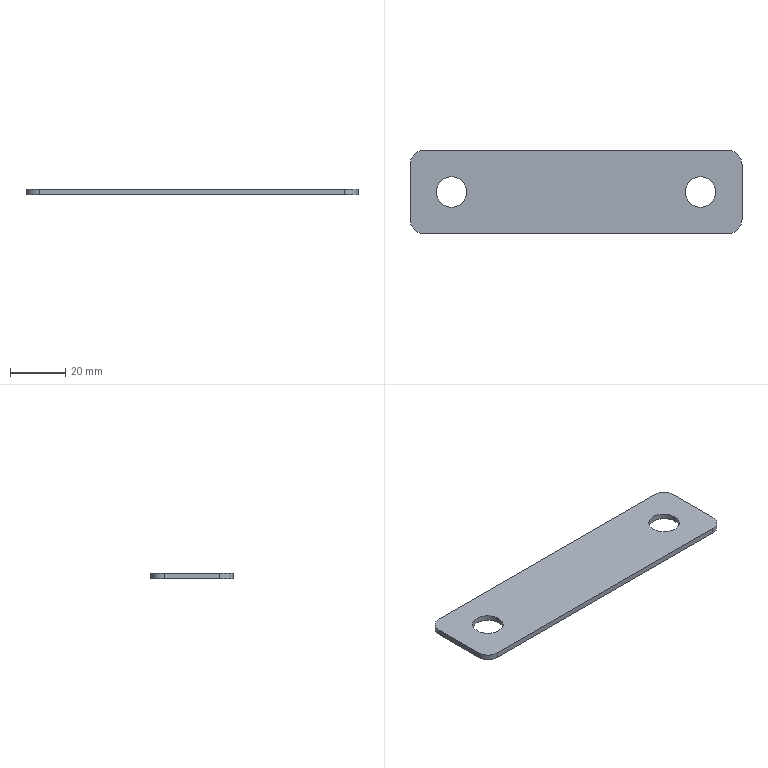Part | SolidWorks | features Extrusion 1, Fillet 1, ICE 1 | 1 solid | 14 faces | box 120 x 30 x 2 mm | volume 6777 mm3 | cylinder 8 | plane 6 | commonest cylinder face diameters 10 x4 11 x4
STEP:
#1=CARTESIAN_POINT('',(-39.5,0.,2.));
#2=VERTEX_POINT('',#1);
#3=CARTESIAN_POINT('',(-50.5,0.,2.));
#4=VERTEX_POINT('',#3);
#5=CARTESIAN_POINT('',(-45.,0.,2.));
#6=DIRECTION('',(0.,0.,-1.));
#7=DIRECTION('',(-1.,0.,0.));
#8=AXIS2_PLACEMENT_3D('',#5,#6,#7);
#9=CIRCLE('',#8,5.5);
#10=EDGE_CURVE('',#2,#4,#9,.T.);
#11=ORIENTED_EDGE('',*,*,#10,.F.);
#12=CARTESIAN_POINT('',(-39.5,0.,0.));
#13=VERTEX_POINT('',#12);
#14=CARTESIAN_POINT('',(-39.5,0.,10.));
#15=DIRECTION('',(0.,0.,-1.));
#16=VECTOR('',#15,1000.);
#17=LINE('',#14,#16);
#18=EDGE_CURVE('',#2,#13,#17,.T.);
#19=ORIENTED_EDGE('',*,*,#18,.T.);
#20=CARTESIAN_POINT('',(-50.5,0.,0.));
#21=VERTEX_POINT('',#20);
#22=CARTESIAN_POINT('',(-45.,0.,0.));
#23=DIRECTION('',(0.,0.,-1.));
#24=DIRECTION('',(-1.,0.,0.));
#25=AXIS2_PLACEMENT_3D('',#22,#23,#24);
#26=CIRCLE('',#25,5.5);
#27=EDGE_CURVE('',#13,#21,#26,.T.);
#28=ORIENTED_EDGE('',*,*,#27,.T.);
#29=CARTESIAN_POINT('',(-50.5,0.,10.));
#30=DIRECTION('',(0.,0.,-1.));
#31=VECTOR('',#30,1000.);
#32=LINE('',#29,#31);
#33=EDGE_CURVE('',#4,#21,#32,.T.);
#34=ORIENTED_EDGE('',*,*,#33,.F.);
#35=EDGE_LOOP('',(#11,#19,#28,#34));
#36=FACE_OUTER_BOUND('',#35,.T.);
#37=CARTESIAN_POINT('',(-45.,0.,10.));
#38=DIRECTION('',(0.,0.,-1.));
#39=DIRECTION('',(-1.,0.,0.));
#40=AXIS2_PLACEMENT_3D('',#37,#38,#39);
#41=CYLINDRICAL_SURFACE('',#40,5.5);
#42=ADVANCED_FACE('',(#36),#41,.F.);
#43=CARTESIAN_POINT('',(50.5,0.,2.));
#44=VERTEX_POINT('',#43);
#45=CARTESIAN_POINT('',(39.5,0.,2.));
#46=VERTEX_POINT('',#45);
#47=CARTESIAN_POINT('',(45.,0.,2.));
#48=DIRECTION('',(0.,0.,-1.));
#49=DIRECTION('',(-1.,0.,0.));
#50=AXIS2_PLACEMENT_3D('',#47,#48,#49);
#51=CIRCLE('',#50,5.5);
#52=EDGE_CURVE('',#44,#46,#51,.T.);
#53=ORIENTED_EDGE('',*,*,#52,.F.);
#54=CARTESIAN_POINT('',(50.5,0.,0.));
#55=VERTEX_POINT('',#54);
#56=CARTESIAN_POINT('',(50.5,0.,10.));
#57=DIRECTION('',(0.,0.,-1.));
#58=VECTOR('',#57,1000.);
#59=LINE('',#56,#58);
#60=EDGE_CURVE('',#44,#55,#59,.T.);
#61=ORIENTED_EDGE('',*,*,#60,.T.);
#62=CARTESIAN_POINT('',(39.5,0.,0.));
#63=VERTEX_POINT('',#62);
#64=CARTESIAN_POINT('',(45.,0.,0.));
#65=DIRECTION('',(0.,0.,-1.));
#66=DIRECTION('',(1.,0.,0.));
#67=AXIS2_PLACEMENT_3D('',#64,#65,#66);
#68=CIRCLE('',#67,5.5);
#69=EDGE_CURVE('',#55,#63,#68,.T.);
#70=ORIENTED_EDGE('',*,*,#69,.T.);
#71=CARTESIAN_POINT('',(39.5,0.,10.));
#72=DIRECTION('',(0.,0.,-1.));
#73=VECTOR('',#72,1000.);
#74=LINE('',#71,#73);
#75=EDGE_CURVE('',#46,#63,#74,.T.);
#76=ORIENTED_EDGE('',*,*,#75,.F.);
#77=EDGE_LOOP('',(#53,#61,#70,#76));
#78=FACE_OUTER_BOUND('',#77,.T.);
#79=CARTESIAN_POINT('',(45.,0.,10.));
#80=DIRECTION('',(0.,0.,-1.));
#81=DIRECTION('',(-1.,0.,0.));
#82=AXIS2_PLACEMENT_3D('',#79,#80,#81);
#83=CYLINDRICAL_SURFACE('',#82,5.5);
#84=ADVANCED_FACE('',(#78),#83,.F.);
#85=CARTESIAN_POINT('',(60.,-10.,2.));
#86=VERTEX_POINT('',#85);
#87=CARTESIAN_POINT('',(60.,10.,2.));
#88=VERTEX_POINT('',#87);
#89=CARTESIAN_POINT('',(60.,-15.,2.));
#90=DIRECTION('',(0.,1.,0.));
#91=VECTOR('',#90,1000.);
#92=LINE('',#89,#91);
#93=EDGE_CURVE('',#86,#88,#92,.T.);
#94=ORIENTED_EDGE('',*,*,#93,.F.);
#95=CARTESIAN_POINT('',(60.,-10.,0.));
#96=VERTEX_POINT('',#95);
#97=CARTESIAN_POINT('',(60.,-10.,2.));
#98=DIRECTION('',(0.,0.,-1.));
#99=VECTOR('',#98,1000.);
#100=LINE('',#97,#99);
#101=EDGE_CURVE('',#86,#96,#100,.T.);
#102=ORIENTED_EDGE('',*,*,#101,.T.);
#103=CARTESIAN_POINT('',(60.,10.,0.));
#104=VERTEX_POINT('',#103);
#105=CARTESIAN_POINT('',(60.,-15.,0.));
#106=DIRECTION('',(0.,1.,0.));
#107=VECTOR('',#106,1000.);
#108=LINE('',#105,#107);
#109=EDGE_CURVE('',#96,#104,#108,.T.);
#110=ORIENTED_EDGE('',*,*,#109,.T.);
#111=CARTESIAN_POINT('',(60.,10.,2.));
#112=DIRECTION('',(0.,0.,1.));
#113=VECTOR('',#112,1000.);
#114=LINE('',#111,#113);
#115=EDGE_CURVE('',#104,#88,#114,.T.);
#116=ORIENTED_EDGE('',*,*,#115,.T.);
#117=EDGE_LOOP('',(#94,#102,#110,#116));
#118=FACE_OUTER_BOUND('',#117,.T.);
#119=CARTESIAN_POINT('',(60.,-15.,2.));
#120=DIRECTION('',(-1.,0.,0.));
#121=DIRECTION('',(0.,0.,1.));
#122=AXIS2_PLACEMENT_3D('',#119,#120,#121);
#123=PLANE('',#122);
#124=ADVANCED_FACE('',(#118),#123,.F.);
#125=CARTESIAN_POINT('',(55.,15.,0.));
#126=VERTEX_POINT('',#125);
#127=CARTESIAN_POINT('',(-55.,15.,0.));
#128=VERTEX_POINT('',#127);
#129=CARTESIAN_POINT('',(-60.,15.,0.));
#130=DIRECTION('',(-1.,0.,0.));
#131=VECTOR('',#130,1000.);
#132=LINE('',#129,#131);
#133=EDGE_CURVE('',#126,#128,#132,.T.);
#134=ORIENTED_EDGE('',*,*,#133,.T.);
#135=CARTESIAN_POINT('',(-55.,15.,2.));
#136=VERTEX_POINT('',#135);
#137=CARTESIAN_POINT('',(-55.,15.,2.));
#138=DIRECTION('',(0.,0.,1.));
#139=VECTOR('',#138,1000.);
#140=LINE('',#137,#139);
#141=EDGE_CURVE('',#128,#136,#140,.T.);
#142=ORIENTED_EDGE('',*,*,#141,.T.);
#143=CARTESIAN_POINT('',(55.,15.,2.));
#144=VERTEX_POINT('',#143);
#145=CARTESIAN_POINT('',(-60.,15.,2.));
#146=DIRECTION('',(-1.,0.,0.));
#147=VECTOR('',#146,1000.);
#148=LINE('',#145,#147);
#149=EDGE_CURVE('',#144,#136,#148,.T.);
#150=ORIENTED_EDGE('',*,*,#149,.F.);
#151=CARTESIAN_POINT('',(55.,15.,2.));
#152=DIRECTION('',(0.,0.,-1.));
#153=VECTOR('',#152,1000.);
#154=LINE('',#151,#153);
#155=EDGE_CURVE('',#144,#126,#154,.T.);
#156=ORIENTED_EDGE('',*,*,#155,.T.);
#157=EDGE_LOOP('',(#134,#142,#150,#156));
#158=FACE_OUTER_BOUND('',#157,.T.);
#159=CARTESIAN_POINT('',(-60.,15.,2.));
#160=DIRECTION('',(0.,-1.,0.));
#161=DIRECTION('',(0.,0.,-1.));
#162=AXIS2_PLACEMENT_3D('',#159,#160,#161);
#163=PLANE('',#162);
#164=ADVANCED_FACE('',(#158),#163,.F.);
#165=CARTESIAN_POINT('',(-60.,10.,0.));
#166=VERTEX_POINT('',#165);
#167=CARTESIAN_POINT('',(-60.,-10.,0.));
#168=VERTEX_POINT('',#167);
#169=CARTESIAN_POINT('',(-60.,-15.,0.));
#170=DIRECTION('',(0.,-1.,0.));
#171=VECTOR('',#170,1000.);
#172=LINE('',#169,#171);
#173=EDGE_CURVE('',#166,#168,#172,.T.);
#174=ORIENTED_EDGE('',*,*,#173,.T.);
#175=CARTESIAN_POINT('',(-60.,-10.,2.));
#176=VERTEX_POINT('',#175);
#177=CARTESIAN_POINT('',(-60.,-10.,2.));
#178=DIRECTION('',(0.,0.,1.));
#179=VECTOR('',#178,1000.);
#180=LINE('',#177,#179);
#181=EDGE_CURVE('',#168,#176,#180,.T.);
#182=ORIENTED_EDGE('',*,*,#181,.T.);
#183=CARTESIAN_POINT('',(-60.,10.,2.));
#184=VERTEX_POINT('',#183);
#185=CARTESIAN_POINT('',(-60.,-15.,2.));
#186=DIRECTION('',(0.,-1.,0.));
#187=VECTOR('',#186,1000.);
#188=LINE('',#185,#187);
#189=EDGE_CURVE('',#184,#176,#188,.T.);
#190=ORIENTED_EDGE('',*,*,#189,.F.);
#191=CARTESIAN_POINT('',(-60.,10.,2.));
#192=DIRECTION('',(0.,0.,-1.));
#193=VECTOR('',#192,1000.);
#194=LINE('',#191,#193);
#195=EDGE_CURVE('',#184,#166,#194,.T.);
#196=ORIENTED_EDGE('',*,*,#195,.T.);
#197=EDGE_LOOP('',(#174,#182,#190,#196));
#198=FACE_OUTER_BOUND('',#197,.T.);
#199=CARTESIAN_POINT('',(-60.,-15.,2.));
#200=DIRECTION('',(1.,0.,0.));
#201=DIRECTION('',(0.,0.,-1.));
#202=AXIS2_PLACEMENT_3D('',#199,#200,#201);
#203=PLANE('',#202);
#204=ADVANCED_FACE('',(#198),#203,.F.);
#205=CARTESIAN_POINT('',(-55.,-15.,2.));
#206=VERTEX_POINT('',#205);
#207=CARTESIAN_POINT('',(55.,-15.,2.));
#208=VERTEX_POINT('',#207);
#209=CARTESIAN_POINT('',(-60.,-15.,2.));
#210=DIRECTION('',(1.,0.,0.));
#211=VECTOR('',#210,1000.);
#212=LINE('',#209,#211);
#213=EDGE_CURVE('',#206,#208,#212,.T.);
#214=ORIENTED_EDGE('',*,*,#213,.F.);
#215=CARTESIAN_POINT('',(-55.,-15.,0.));
#216=VERTEX_POINT('',#215);
#217=CARTESIAN_POINT('',(-55.,-15.,2.));
#218=DIRECTION('',(0.,0.,-1.));
#219=VECTOR('',#218,1000.);
#220=LINE('',#217,#219);
#221=EDGE_CURVE('',#206,#216,#220,.T.);
#222=ORIENTED_EDGE('',*,*,#221,.T.);
#223=CARTESIAN_POINT('',(55.,-15.,0.));
#224=VERTEX_POINT('',#223);
#225=CARTESIAN_POINT('',(-60.,-15.,0.));
#226=DIRECTION('',(1.,0.,0.));
#227=VECTOR('',#226,1000.);
#228=LINE('',#225,#227);
#229=EDGE_CURVE('',#216,#224,#228,.T.);
#230=ORIENTED_EDGE('',*,*,#229,.T.);
#231=CARTESIAN_POINT('',(55.,-15.,2.));
#232=DIRECTION('',(0.,0.,1.));
#233=VECTOR('',#232,1000.);
#234=LINE('',#231,#233);
#235=EDGE_CURVE('',#224,#208,#234,.T.);
#236=ORIENTED_EDGE('',*,*,#235,.T.);
#237=EDGE_LOOP('',(#214,#222,#230,#236));
#238=FACE_OUTER_BOUND('',#237,.T.);
#239=CARTESIAN_POINT('',(-60.,-15.,2.));
#240=DIRECTION('',(0.,1.,0.));
#241=DIRECTION('',(0.,0.,1.));
#242=AXIS2_PLACEMENT_3D('',#239,#240,#241);
#243=PLANE('',#242);
#244=ADVANCED_FACE('',(#238),#243,.F.);
#245=CARTESIAN_POINT('',(-45.,0.,2.));
#246=DIRECTION('',(0.,0.,-1.));
#247=DIRECTION('',(-1.,0.,0.));
#248=AXIS2_PLACEMENT_3D('',#245,#246,#247);
#249=CIRCLE('',#248,5.5);
#250=EDGE_CURVE('',#4,#2,#249,.T.);
#251=ORIENTED_EDGE('',*,*,#250,.T.);
#252=ORIENTED_EDGE('',*,*,#10,.T.);
#253=EDGE_LOOP('',(#251,#252));
#254=FACE_BOUND('',#253,.T.);
#255=CARTESIAN_POINT('',(45.,0.,2.));
#256=DIRECTION('',(0.,0.,-1.));
#257=DIRECTION('',(-1.,0.,0.));
#258=AXIS2_PLACEMENT_3D('',#255,#256,#257);
#259=CIRCLE('',#258,5.5);
#260=EDGE_CURVE('',#46,#44,#259,.T.);
#261=ORIENTED_EDGE('',*,*,#260,.T.);
#262=ORIENTED_EDGE('',*,*,#52,.T.);
#263=EDGE_LOOP('',(#261,#262));
#264=FACE_BOUND('',#263,.T.);
#265=ORIENTED_EDGE('',*,*,#189,.T.);
#266=CARTESIAN_POINT('',(-55.,-10.,2.));
#267=DIRECTION('',(0.,0.,1.));
#268=DIRECTION('',(-1.,0.,0.));
#269=AXIS2_PLACEMENT_3D('',#266,#267,#268);
#270=CIRCLE('',#269,5.);
#271=EDGE_CURVE('',#176,#206,#270,.T.);
#272=ORIENTED_EDGE('',*,*,#271,.T.);
#273=ORIENTED_EDGE('',*,*,#213,.T.);
#274=CARTESIAN_POINT('',(55.,-10.,2.));
#275=DIRECTION('',(0.,0.,1.));
#276=DIRECTION('',(-1.,0.,0.));
#277=AXIS2_PLACEMENT_3D('',#274,#275,#276);
#278=CIRCLE('',#277,5.);
#279=EDGE_CURVE('',#208,#86,#278,.T.);
#280=ORIENTED_EDGE('',*,*,#279,.T.);
#281=ORIENTED_EDGE('',*,*,#93,.T.);
#282=CARTESIAN_POINT('',(55.,10.,2.));
#283=DIRECTION('',(0.,0.,1.));
#284=DIRECTION('',(-1.,0.,0.));
#285=AXIS2_PLACEMENT_3D('',#282,#283,#284);
#286=CIRCLE('',#285,5.);
#287=EDGE_CURVE('',#88,#144,#286,.T.);
#288=ORIENTED_EDGE('',*,*,#287,.T.);
#289=ORIENTED_EDGE('',*,*,#149,.T.);
#290=CARTESIAN_POINT('',(-55.,10.,2.));
#291=DIRECTION('',(0.,0.,1.));
#292=DIRECTION('',(-1.,0.,0.));
#293=AXIS2_PLACEMENT_3D('',#290,#291,#292);
#294=CIRCLE('',#293,5.);
#295=EDGE_CURVE('',#136,#184,#294,.T.);
#296=ORIENTED_EDGE('',*,*,#295,.T.);
#297=EDGE_LOOP('',(#265,#272,#273,#280,#281,#288,#289,#296));
#298=FACE_OUTER_BOUND('',#297,.T.);
#299=CARTESIAN_POINT('',(0.,0.,2.));
#300=DIRECTION('',(0.,0.,-1.));
#301=DIRECTION('',(-1.,0.,0.));
#302=AXIS2_PLACEMENT_3D('',#299,#300,#301);
#303=PLANE('',#302);
#304=ADVANCED_FACE('',(#254,#264,#298),#303,.F.);
#305=CARTESIAN_POINT('',(-45.,0.,0.));
#306=DIRECTION('',(0.,0.,-1.));
#307=DIRECTION('',(-1.,0.,0.));
#308=AXIS2_PLACEMENT_3D('',#305,#306,#307);
#309=CIRCLE('',#308,5.5);
#310=EDGE_CURVE('',#21,#13,#309,.T.);
#311=ORIENTED_EDGE('',*,*,#310,.F.);
#312=ORIENTED_EDGE('',*,*,#27,.F.);
#313=EDGE_LOOP('',(#311,#312));
#314=FACE_BOUND('',#313,.T.);
#315=CARTESIAN_POINT('',(45.,0.,0.));
#316=DIRECTION('',(0.,0.,-1.));
#317=DIRECTION('',(1.,0.,0.));
#318=AXIS2_PLACEMENT_3D('',#315,#316,#317);
#319=CIRCLE('',#318,5.5);
#320=EDGE_CURVE('',#63,#55,#319,.T.);
#321=ORIENTED_EDGE('',*,*,#320,.F.);
#322=ORIENTED_EDGE('',*,*,#69,.F.);
#323=EDGE_LOOP('',(#321,#322));
#324=FACE_BOUND('',#323,.T.);
#325=ORIENTED_EDGE('',*,*,#229,.F.);
#326=CARTESIAN_POINT('',(-55.,-10.,0.));
#327=DIRECTION('',(0.,0.,-1.));
#328=DIRECTION('',(-1.,0.,0.));
#329=AXIS2_PLACEMENT_3D('',#326,#327,#328);
#330=CIRCLE('',#329,5.);
#331=EDGE_CURVE('',#216,#168,#330,.T.);
#332=ORIENTED_EDGE('',*,*,#331,.T.);
#333=ORIENTED_EDGE('',*,*,#173,.F.);
#334=CARTESIAN_POINT('',(-55.,10.,0.));
#335=DIRECTION('',(0.,0.,-1.));
#336=DIRECTION('',(-1.,0.,0.));
#337=AXIS2_PLACEMENT_3D('',#334,#335,#336);
#338=CIRCLE('',#337,5.);
#339=EDGE_CURVE('',#166,#128,#338,.T.);
#340=ORIENTED_EDGE('',*,*,#339,.T.);
#341=ORIENTED_EDGE('',*,*,#133,.F.);
#342=CARTESIAN_POINT('',(55.,10.,0.));
#343=DIRECTION('',(0.,0.,-1.));
#344=DIRECTION('',(-1.,0.,0.));
#345=AXIS2_PLACEMENT_3D('',#342,#343,#344);
#346=CIRCLE('',#345,5.);
#347=EDGE_CURVE('',#126,#104,#346,.T.);
#348=ORIENTED_EDGE('',*,*,#347,.T.);
#349=ORIENTED_EDGE('',*,*,#109,.F.);
#350=CARTESIAN_POINT('',(55.,-10.,0.));
#351=DIRECTION('',(0.,0.,-1.));
#352=DIRECTION('',(-1.,0.,0.));
#353=AXIS2_PLACEMENT_3D('',#350,#351,#352);
#354=CIRCLE('',#353,5.);
#355=EDGE_CURVE('',#96,#224,#354,.T.);
#356=ORIENTED_EDGE('',*,*,#355,.T.);
#357=EDGE_LOOP('',(#325,#332,#333,#340,#341,#348,#349,#356));
#358=FACE_OUTER_BOUND('',#357,.T.);
#359=CARTESIAN_POINT('',(0.,0.,0.));
#360=DIRECTION('',(0.,0.,-1.));
#361=DIRECTION('',(-1.,0.,0.));
#362=AXIS2_PLACEMENT_3D('',#359,#360,#361);
#363=PLANE('',#362);
#364=ADVANCED_FACE('',(#314,#324,#358),#363,.T.);
#365=ORIENTED_EDGE('',*,*,#60,.F.);
#366=ORIENTED_EDGE('',*,*,#260,.F.);
#367=ORIENTED_EDGE('',*,*,#75,.T.);
#368=ORIENTED_EDGE('',*,*,#320,.T.);
#369=EDGE_LOOP('',(#365,#366,#367,#368));
#370=FACE_OUTER_BOUND('',#369,.T.);
#371=CARTESIAN_POINT('',(45.,0.,10.));
#372=DIRECTION('',(0.,0.,-1.));
#373=DIRECTION('',(-1.,0.,0.));
#374=AXIS2_PLACEMENT_3D('',#371,#372,#373);
#375=CYLINDRICAL_SURFACE('',#374,5.5);
#376=ADVANCED_FACE('',(#370),#375,.F.);
#377=ORIENTED_EDGE('',*,*,#18,.F.);
#378=ORIENTED_EDGE('',*,*,#250,.F.);
#379=ORIENTED_EDGE('',*,*,#33,.T.);
#380=ORIENTED_EDGE('',*,*,#310,.T.);
#381=EDGE_LOOP('',(#377,#378,#379,#380));
#382=FACE_OUTER_BOUND('',#381,.T.);
#383=CARTESIAN_POINT('',(-45.,0.,10.));
#384=DIRECTION('',(0.,0.,-1.));
#385=DIRECTION('',(-1.,0.,0.));
#386=AXIS2_PLACEMENT_3D('',#383,#384,#385);
#387=CYLINDRICAL_SURFACE('',#386,5.5);
#388=ADVANCED_FACE('',(#382),#387,.F.);
#389=ORIENTED_EDGE('',*,*,#271,.F.);
#390=ORIENTED_EDGE('',*,*,#181,.F.);
#391=ORIENTED_EDGE('',*,*,#331,.F.);
#392=ORIENTED_EDGE('',*,*,#221,.F.);
#393=EDGE_LOOP('',(#389,#390,#391,#392));
#394=FACE_OUTER_BOUND('',#393,.T.);
#395=CARTESIAN_POINT('',(-55.,-10.,2.));
#396=DIRECTION('',(0.,0.,-1.));
#397=DIRECTION('',(-1.,0.,0.));
#398=AXIS2_PLACEMENT_3D('',#395,#396,#397);
#399=CYLINDRICAL_SURFACE('',#398,5.);
#400=ADVANCED_FACE('',(#394),#399,.T.);
#401=ORIENTED_EDGE('',*,*,#295,.F.);
#402=ORIENTED_EDGE('',*,*,#141,.F.);
#403=ORIENTED_EDGE('',*,*,#339,.F.);
#404=ORIENTED_EDGE('',*,*,#195,.F.);
#405=EDGE_LOOP('',(#401,#402,#403,#404));
#406=FACE_OUTER_BOUND('',#405,.T.);
#407=CARTESIAN_POINT('',(-55.,10.,2.));
#408=DIRECTION('',(0.,0.,-1.));
#409=DIRECTION('',(-1.,0.,0.));
#410=AXIS2_PLACEMENT_3D('',#407,#408,#409);
#411=CYLINDRICAL_SURFACE('',#410,5.);
#412=ADVANCED_FACE('',(#406),#411,.T.);
#413=ORIENTED_EDGE('',*,*,#279,.F.);
#414=ORIENTED_EDGE('',*,*,#235,.F.);
#415=ORIENTED_EDGE('',*,*,#355,.F.);
#416=ORIENTED_EDGE('',*,*,#101,.F.);
#417=EDGE_LOOP('',(#413,#414,#415,#416));
#418=FACE_OUTER_BOUND('',#417,.T.);
#419=CARTESIAN_POINT('',(55.,-10.,2.));
#420=DIRECTION('',(0.,0.,-1.));
#421=DIRECTION('',(-1.,0.,0.));
#422=AXIS2_PLACEMENT_3D('',#419,#420,#421);
#423=CYLINDRICAL_SURFACE('',#422,5.);
#424=ADVANCED_FACE('',(#418),#423,.T.);
#425=ORIENTED_EDGE('',*,*,#287,.F.);
#426=ORIENTED_EDGE('',*,*,#115,.F.);
#427=ORIENTED_EDGE('',*,*,#347,.F.);
#428=ORIENTED_EDGE('',*,*,#155,.F.);
#429=EDGE_LOOP('',(#425,#426,#427,#428));
#430=FACE_OUTER_BOUND('',#429,.T.);
#431=CARTESIAN_POINT('',(55.,10.,2.));
#432=DIRECTION('',(0.,0.,-1.));
#433=DIRECTION('',(-1.,0.,0.));
#434=AXIS2_PLACEMENT_3D('',#431,#432,#433);
#435=CYLINDRICAL_SURFACE('',#434,5.);
#436=ADVANCED_FACE('',(#430),#435,.T.);
#437=CLOSED_SHELL('',(#42,#84,#124,#164,#204,#244,#304,#364,#376,#388,#400,#412,#424,#436));
#438=MANIFOLD_SOLID_BREP('',#437);
#439=CARTESIAN_POINT('',(0.,0.,0.));
#440=DIRECTION('',(0.,0.,1.));
#441=DIRECTION('',(1.,0.,0.));
#442=AXIS2_PLACEMENT_3D('',#439,#440,#441);
#443=(LENGTH_UNIT()NAMED_UNIT(*)SI_UNIT(.MILLI.,.METRE.));
#444=UNCERTAINTY_MEASURE_WITH_UNIT(LENGTH_MEASURE(0.00001),#443,'','');
#445=(NAMED_UNIT(*)PLANE_ANGLE_UNIT()SI_UNIT($,.RADIAN.));
#446=(NAMED_UNIT(*)SI_UNIT($,.STERADIAN.)SOLID_ANGLE_UNIT());
#447=(GEOMETRIC_REPRESENTATION_CONTEXT(3)GLOBAL_UNCERTAINTY_ASSIGNED_CONTEXT((#444))GLOBAL_UNIT_ASSIGNED_CONTEXT((#443,#445,#446))REPRESENTATION_CONTEXT('',''));
#448=ADVANCED_BREP_SHAPE_REPRESENTATION('',(#438,#442),#447);